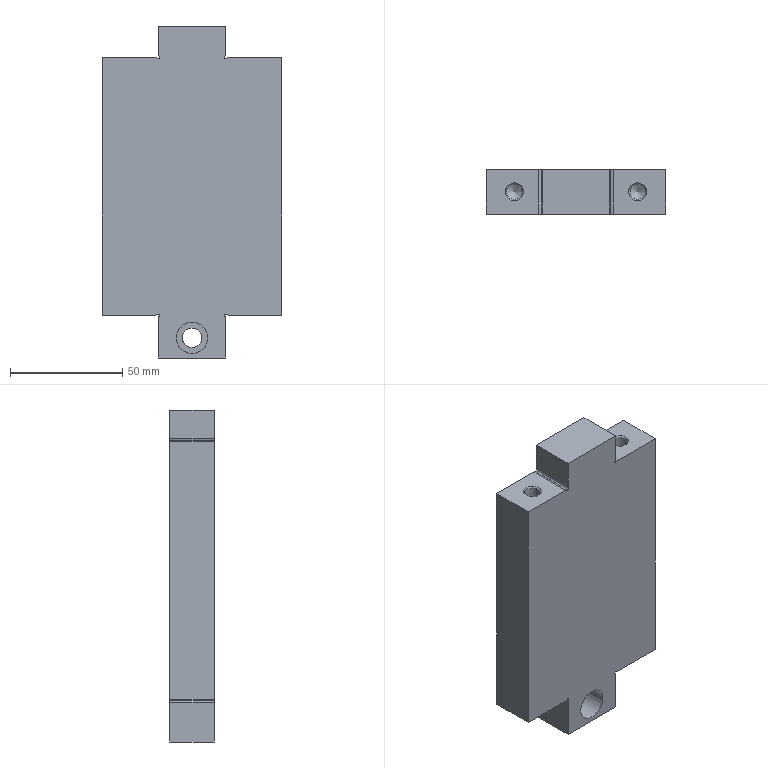Part | STEP file | YBQDJ-YY-3 | 1 solid | 41 faces | box 80 x 20 x 148 mm | volume 197857 mm3 | cylinder 18 | plane 15 | cone 8 | commonest cylinder face diameters 4 x8 1 x4 6.8 x4 8.7 x1 14 x1